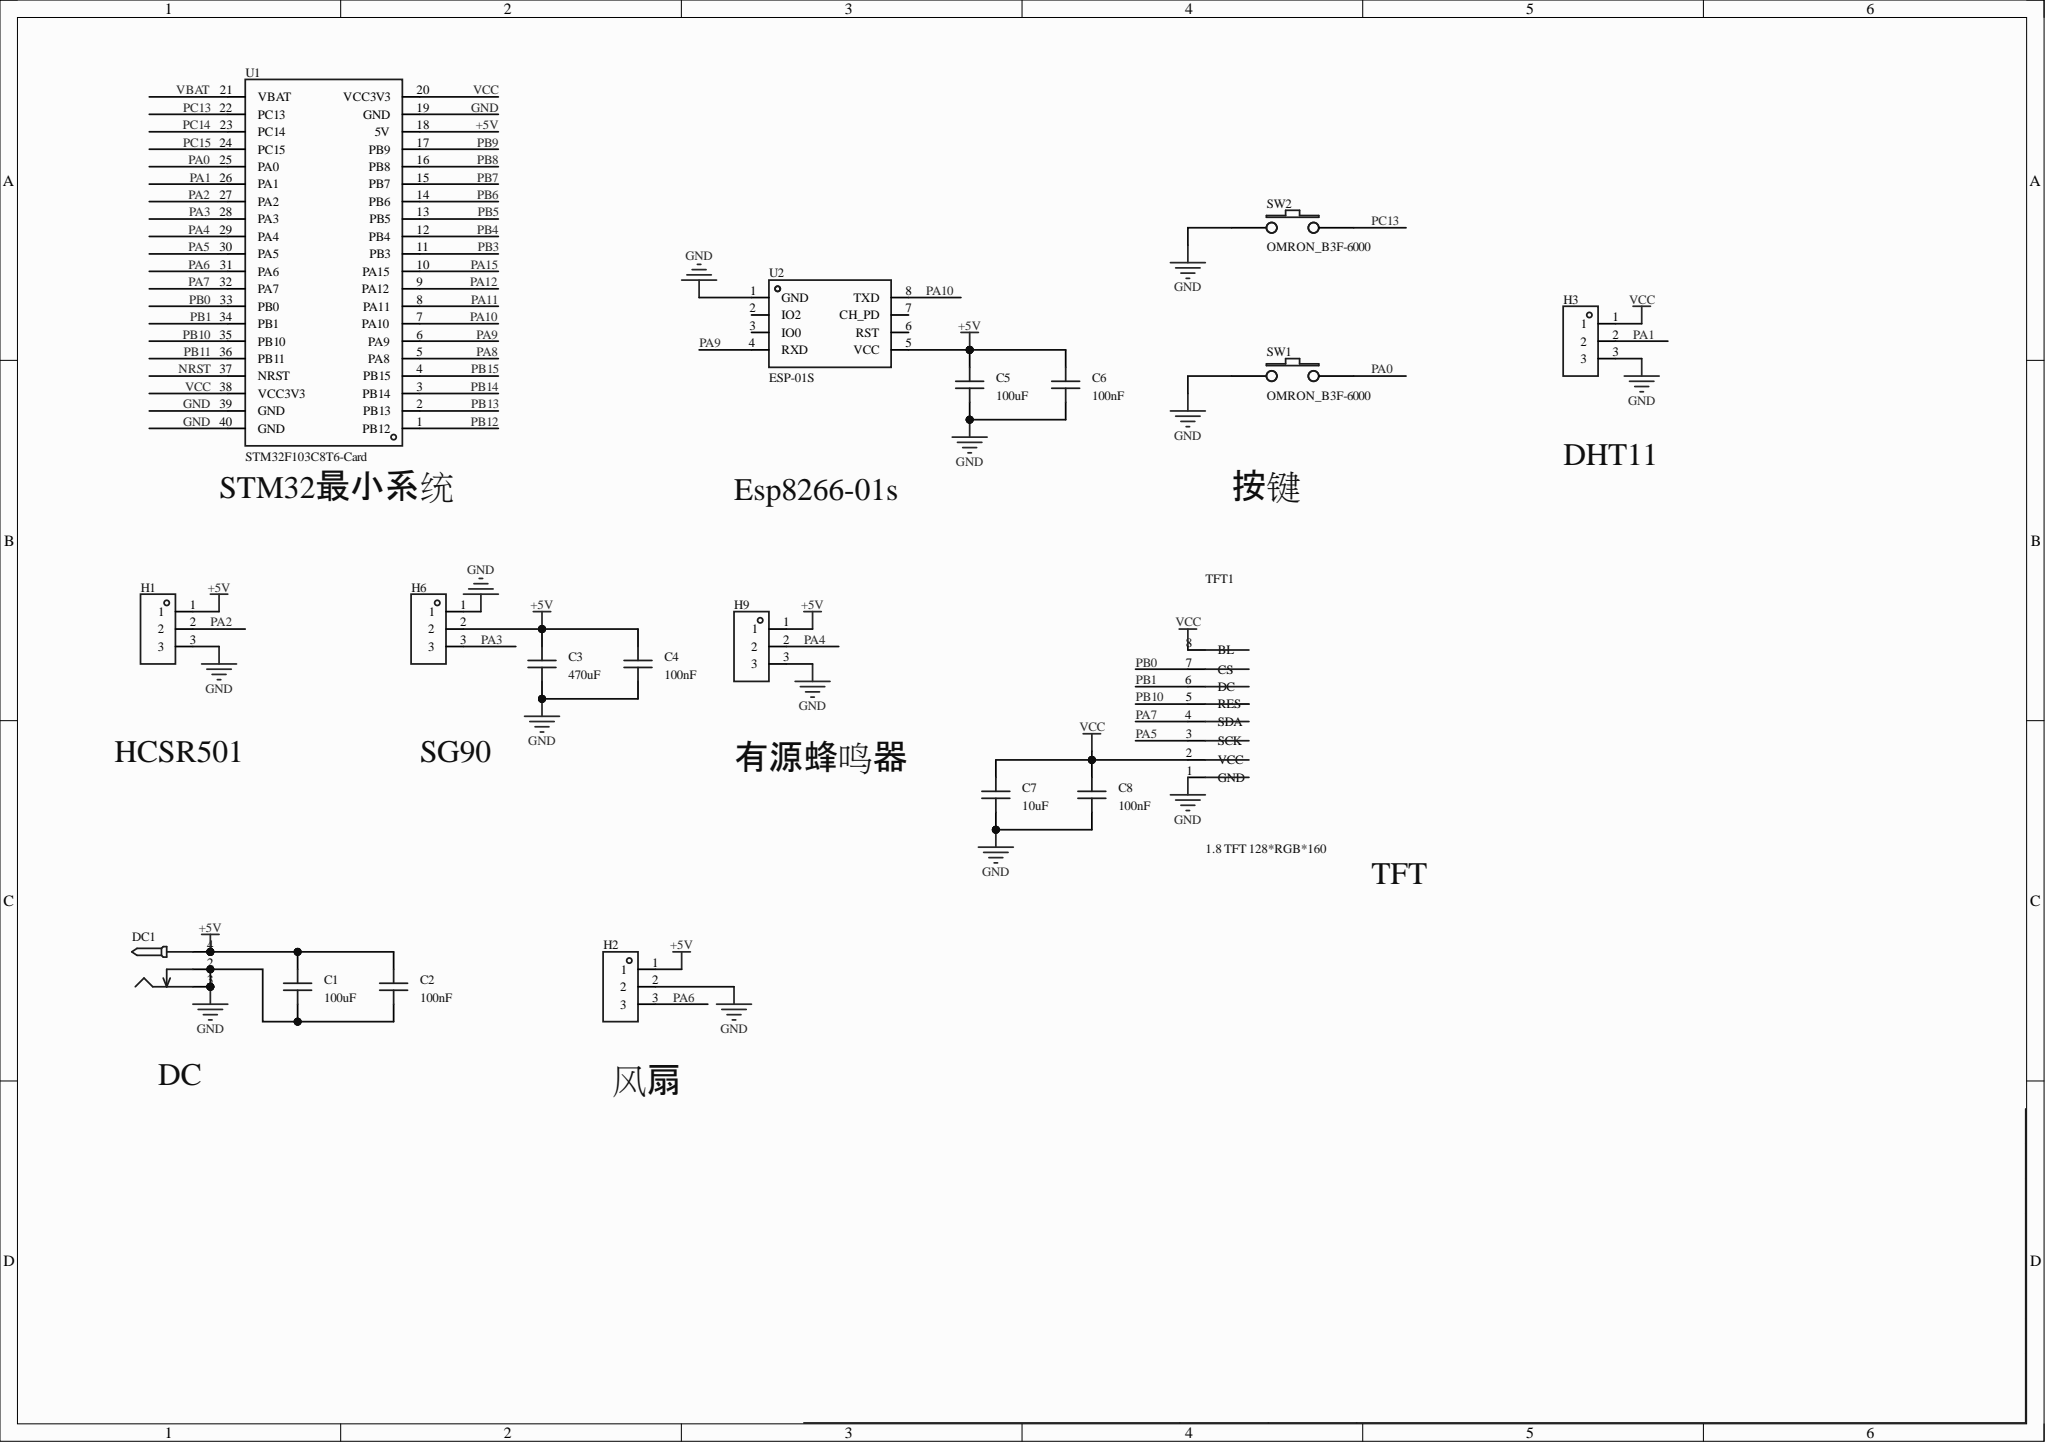Circuit board | Altium Designer | 19 parts | 17 nets
Bill of materials:
Comment,Description,Designator,Footprint,LibRef,Quantity
"100uF","","C1, C5","C0805","CAP_0805","2"
"100nF","","C2, C4, C6, C8","C0805","CAP_0805","4"
"470uF","","C3","C0805","CAP_0805","1"
"10uF","","C7","C0805","CAP_0805","1"
"","","DC1","DC-2.0","DC-005_2.0","1"
"","","H1, H2, H3, H6, H9","HDR-TH_3P-P2.54-V-F","HDR-F_2.54_1x3P","5"
"OMRON_B3F-6000","","SW1, SW2","KEY-TH_2P-L6.0-W6.0-P5.00","OMRON_B3F-6000","2"
"1.8 TFT 128*RGB*160","","TFT1","LCD-TH_8P-P2.54-L56.0-W34.0_1.8-TFT","1.8 TFT 128*RGB*160","1"
"STM32F103C8T6-Card","","U1","CONN-TH_L53.3-W22.9_STM32F103C8T6-CARD","STM32F103C8T6-Card","1"
"ESP-01S","","U2","WIFIM-TH_ESP-01S","ESP-01S_C111009","1"
Netlist (Protel format):
[
C1
C0805
100uF



]
[
C2
C0805
100nF



]
[
C3
C0805
470uF



]
[
C4
C0805
100nF



]
[
C5
C0805
100uF



]
[
C6
C0805
100nF



]
[
C7
C0805
10uF



]
[
C8
C0805
100nF



]
[
DC1
DC-2.0




]
[
H1
HDR-TH_3P-P2.54-V-F




]
[
H2
HDR-TH_3P-P2.54-V-F




]
[
H3
HDR-TH_3P-P2.54-V-F




]
[
H6
HDR-TH_3P-P2.54-V-F




]
[
H9
HDR-TH_3P-P2.54-V-F




]
[
SW1
KEY-TH_2P-L6.0-W6.0-P5.00
OMRON_B3F-6000



]
[
SW2
KEY-TH_2P-L6.0-W6.0-P5.00
OMRON_B3F-6000



]
[
TFT1
LCD-TH_8P-P2.54-L56.0-W34.0_1.8-TFT
1.8 TFT 128*RGB*160



]
[
U1
CONN-TH_L53.3-W22.9_STM32F103C8T6-CARD
STM32F103C8T6-Card



]
[
U2
WIFIM-TH_ESP-01S
ESP-01S



]
(
VCC
C7-2
C8-2
H3-1
TFT1-2
TFT1-8
U1-20
U1-38
)
(
PC13
SW2-2
U1-22
)
(
PB10
TFT1-5
U1-35
)
(
PB1
TFT1-6
U1-34
)
(
PB0
TFT1-7
U1-33
)
(
PA10
U1-7
U2-8
)
(
PA9
U1-6
U2-4
)
(
PA7
TFT1-4
U1-32
)
(
PA6
H2-3
U1-31
)
(
PA5
TFT1-3
U1-30
)
(
PA4
H9-2
U1-29
)
(
PA3
H6-3
U1-28
)
(
PA2
H1-2
U1-27
)
(
PA1
H3-2
U1-26
)
(
PA0
SW1-2
U1-25
)
(
GND
C1-1
C2-1
C3-1
C4-1
C5-1
C6-1
C7-1
C8-1
DC1-2
DC1-3
H1-3
H2-2
H3-3
H6-1
H9-3
SW1-1
SW2-1
TFT1-1
U1-19
U1-39
U1-40
U2-1
)
(
+5V
C1-2
C2-2
C3-2
C4-2
C5-2
C6-2
DC1-4
H1-1
H2-1
H6-2
H9-1
U1-18
U2-5
)